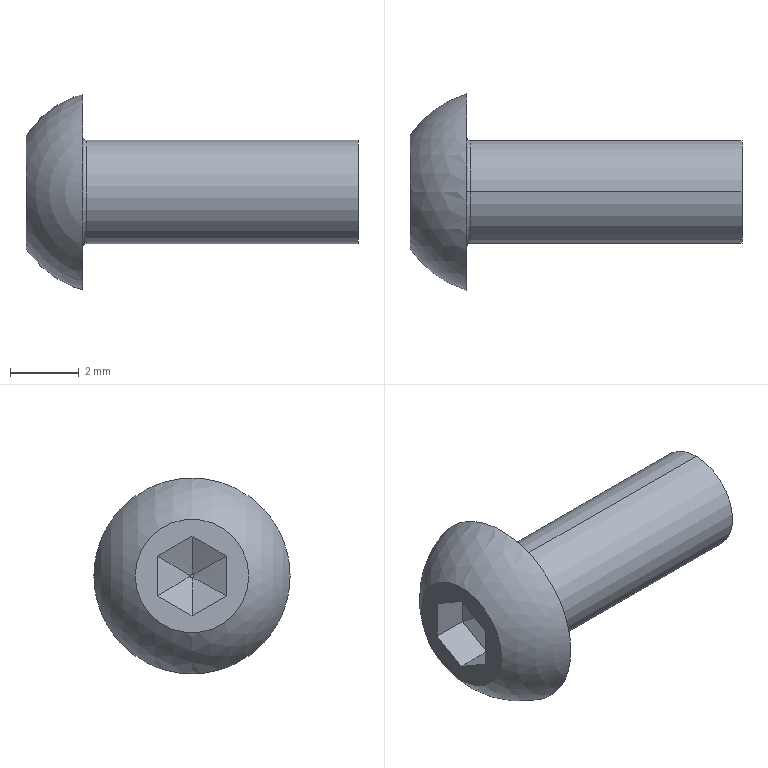Part | NX | features BREP 1 | 1 solid | 21 faces | box 9.65 x 5.7 x 5.7 mm | volume 82.821 mm3 | plane 10 | spline 6 | torus 2 | cylinder 2 | sphere 1 | commonest cylinder face diameters 3 x2
STEP:
#1=CARTESIAN_POINT('',(1.75,0.,1.5));
#2=VERTEX_POINT('',#1);
#3=CARTESIAN_POINT('',(1.75,0.,-1.5));
#4=VERTEX_POINT('',#3);
#5=CARTESIAN_POINT('',(1.75,0.,0.));
#6=DIRECTION('',(1.,0.,0.));
#7=DIRECTION('',(0.,0.,-1.));
#8=AXIS2_PLACEMENT_3D('',#5,#6,#7);
#9=CIRCLE('',#8,1.5);
#10=EDGE_CURVE('',#2,#4,#9,.T.);
#11=ORIENTED_EDGE('',*,*,#10,.F.);
#12=CARTESIAN_POINT('',(1.65,0.,1.6));
#13=VERTEX_POINT('',#12);
#14=CARTESIAN_POINT('',(1.75,0.,1.6));
#15=DIRECTION('',(0.,1.,0.));
#16=DIRECTION('',(0.,0.,1.));
#17=AXIS2_PLACEMENT_3D('',#14,#15,#16);
#18=CIRCLE('',#17,0.1);
#19=EDGE_CURVE('',#13,#2,#18,.F.);
#20=ORIENTED_EDGE('',*,*,#19,.F.);
#21=CARTESIAN_POINT('',(1.65,0.,-1.6));
#22=VERTEX_POINT('',#21);
#23=CARTESIAN_POINT('',(1.65,0.,0.));
#24=DIRECTION('',(-1.,0.,0.));
#25=DIRECTION('',(0.,0.,-1.));
#26=AXIS2_PLACEMENT_3D('',#23,#24,#25);
#27=CIRCLE('',#26,1.6);
#28=EDGE_CURVE('',#22,#13,#27,.T.);
#29=ORIENTED_EDGE('',*,*,#28,.F.);
#30=CARTESIAN_POINT('',(1.75,0.,-1.6));
#31=DIRECTION('',(0.,-1.,0.));
#32=DIRECTION('',(0.,0.,-1.));
#33=AXIS2_PLACEMENT_3D('',#30,#31,#32);
#34=CIRCLE('',#33,0.1);
#35=EDGE_CURVE('',#22,#4,#34,.F.);
#36=ORIENTED_EDGE('',*,*,#35,.T.);
#37=EDGE_LOOP('',(#11,#20,#29,#36));
#38=FACE_BOUND('',#37,.T.);
#39=CARTESIAN_POINT('',(1.75,0.,0.));
#40=DIRECTION('',(1.,0.,0.));
#41=DIRECTION('',(0.,0.,1.));
#42=AXIS2_PLACEMENT_3D('',#39,#40,#41);
#43=TOROIDAL_SURFACE('',#42,1.6,0.1);
#44=ADVANCED_FACE('',(#38),#43,.F.);
#45=CARTESIAN_POINT('',(9.65,0.,1.5));
#46=VERTEX_POINT('',#45);
#47=CARTESIAN_POINT('',(9.65,0.,-1.5));
#48=VERTEX_POINT('',#47);
#49=CARTESIAN_POINT('',(9.65,0.,0.));
#50=DIRECTION('',(-1.,0.,0.));
#51=DIRECTION('',(0.,0.,-1.));
#52=AXIS2_PLACEMENT_3D('',#49,#50,#51);
#53=CIRCLE('',#52,1.5);
#54=EDGE_CURVE('',#46,#48,#53,.T.);
#55=ORIENTED_EDGE('',*,*,#54,.T.);
#56=CARTESIAN_POINT('',(7.65,0.,-1.5));
#57=DIRECTION('',(-1.,0.,0.));
#58=VECTOR('',#57,1000.);
#59=LINE('',#56,#58);
#60=EDGE_CURVE('',#48,#4,#59,.T.);
#61=ORIENTED_EDGE('',*,*,#60,.T.);
#62=CARTESIAN_POINT('',(1.75,0.,0.));
#63=DIRECTION('',(1.,0.,0.));
#64=DIRECTION('',(0.,0.,-1.));
#65=AXIS2_PLACEMENT_3D('',#62,#63,#64);
#66=CIRCLE('',#65,1.5);
#67=EDGE_CURVE('',#4,#2,#66,.T.);
#68=ORIENTED_EDGE('',*,*,#67,.T.);
#69=CARTESIAN_POINT('',(7.65,0.,1.5));
#70=DIRECTION('',(-1.,0.,0.));
#71=VECTOR('',#70,1000.);
#72=LINE('',#69,#71);
#73=EDGE_CURVE('',#46,#2,#72,.T.);
#74=ORIENTED_EDGE('',*,*,#73,.F.);
#75=EDGE_LOOP('',(#55,#61,#68,#74));
#76=FACE_BOUND('',#75,.T.);
#77=CARTESIAN_POINT('',(7.65,0.,0.));
#78=DIRECTION('',(-1.,0.,0.));
#79=DIRECTION('',(0.,0.,-1.));
#80=AXIS2_PLACEMENT_3D('',#77,#78,#79);
#81=CYLINDRICAL_SURFACE('',#80,1.5);
#82=ADVANCED_FACE('',(#76),#81,.T.);
#83=CARTESIAN_POINT('',(1.65,2.85,0.));
#84=VERTEX_POINT('',#83);
#85=CARTESIAN_POINT('',(1.65,-2.85,0.));
#86=VERTEX_POINT('',#85);
#87=CARTESIAN_POINT('',(1.65,0.,0.));
#88=DIRECTION('',(1.,0.,0.));
#89=DIRECTION('',(0.,0.,-1.));
#90=AXIS2_PLACEMENT_3D('',#87,#88,#89);
#91=CIRCLE('',#90,2.85);
#92=EDGE_CURVE('',#84,#86,#91,.T.);
#93=ORIENTED_EDGE('',*,*,#92,.T.);
#94=CARTESIAN_POINT('',(1.65,0.,0.));
#95=DIRECTION('',(1.,0.,0.));
#96=DIRECTION('',(0.,0.,-1.));
#97=AXIS2_PLACEMENT_3D('',#94,#95,#96);
#98=CIRCLE('',#97,2.85);
#99=EDGE_CURVE('',#86,#84,#98,.T.);
#100=ORIENTED_EDGE('',*,*,#99,.T.);
#101=EDGE_LOOP('',(#93,#100));
#102=FACE_BOUND('',#101,.T.);
#103=ORIENTED_EDGE('',*,*,#28,.T.);
#104=CARTESIAN_POINT('',(1.65,0.,0.));
#105=DIRECTION('',(-1.,0.,0.));
#106=DIRECTION('',(0.,0.,-1.));
#107=AXIS2_PLACEMENT_3D('',#104,#105,#106);
#108=CIRCLE('',#107,1.6);
#109=EDGE_CURVE('',#13,#22,#108,.T.);
#110=ORIENTED_EDGE('',*,*,#109,.T.);
#111=EDGE_LOOP('',(#103,#110));
#112=FACE_BOUND('',#111,.T.);
#113=CARTESIAN_POINT('',(1.65,0.,0.));
#114=DIRECTION('',(1.,0.,0.));
#115=DIRECTION('',(0.,-1.,0.));
#116=AXIS2_PLACEMENT_3D('',#113,#114,#115);
#117=PLANE('',#116);
#118=ADVANCED_FACE('',(#102,#112),#117,.T.);
#119=ORIENTED_EDGE('',*,*,#92,.F.);
#120=ORIENTED_EDGE('',*,*,#99,.F.);
#121=EDGE_LOOP('',(#119,#120));
#122=FACE_BOUND('',#121,.T.);
#123=CARTESIAN_POINT('',(0.,1.65,0.));
#124=VERTEX_POINT('',#123);
#125=CARTESIAN_POINT('',(0.,-1.65,0.));
#126=VERTEX_POINT('',#125);
#127=CARTESIAN_POINT('',(0.,0.,0.));
#128=DIRECTION('',(1.,0.,0.));
#129=DIRECTION('',(0.,0.,-1.));
#130=AXIS2_PLACEMENT_3D('',#127,#128,#129);
#131=CIRCLE('',#130,1.65);
#132=EDGE_CURVE('',#124,#126,#131,.T.);
#133=ORIENTED_EDGE('',*,*,#132,.T.);
#134=CARTESIAN_POINT('',(0.,0.,0.));
#135=DIRECTION('',(1.,0.,0.));
#136=DIRECTION('',(0.,0.,-1.));
#137=AXIS2_PLACEMENT_3D('',#134,#135,#136);
#138=CIRCLE('',#137,1.65);
#139=EDGE_CURVE('',#126,#124,#138,.T.);
#140=ORIENTED_EDGE('',*,*,#139,.T.);
#141=EDGE_LOOP('',(#133,#140));
#142=FACE_BOUND('',#141,.T.);
#143=CARTESIAN_POINT('',(2.461,0.,0.));
#144=DIRECTION('',(0.,1.,0.));
#145=DIRECTION('',(-0.2585,0.,-0.966));
#146=AXIS2_PLACEMENT_3D('',#143,#144,#145);
#147=SPHERICAL_SURFACE('',#146,2.963);
#148=ADVANCED_FACE('',(#122,#142),#147,.T.);
#149=ORIENTED_EDGE('',*,*,#132,.F.);
#150=ORIENTED_EDGE('',*,*,#139,.F.);
#151=EDGE_LOOP('',(#149,#150));
#152=FACE_BOUND('',#151,.T.);
#153=CARTESIAN_POINT('',(0.,1.,-0.5774));
#154=VERTEX_POINT('',#153);
#155=CARTESIAN_POINT('',(0.,0.,-1.155));
#156=VERTEX_POINT('',#155);
#157=CARTESIAN_POINT('',(0.,1.,-0.5774));
#158=DIRECTION('',(0.,-0.866,-0.5));
#159=VECTOR('',#158,1000.);
#160=LINE('',#157,#159);
#161=EDGE_CURVE('',#154,#156,#160,.T.);
#162=ORIENTED_EDGE('',*,*,#161,.F.);
#163=CARTESIAN_POINT('',(0.,1.,0.5774));
#164=VERTEX_POINT('',#163);
#165=CARTESIAN_POINT('',(0.,1.,0.));
#166=DIRECTION('',(0.,0.,-1.));
#167=VECTOR('',#166,1000.);
#168=LINE('',#165,#167);
#169=EDGE_CURVE('',#164,#154,#168,.T.);
#170=ORIENTED_EDGE('',*,*,#169,.F.);
#171=CARTESIAN_POINT('',(0.,0.,1.155));
#172=VERTEX_POINT('',#171);
#173=CARTESIAN_POINT('',(0.,0.,1.155));
#174=DIRECTION('',(0.,0.866,-0.5));
#175=VECTOR('',#174,1000.);
#176=LINE('',#173,#175);
#177=EDGE_CURVE('',#172,#164,#176,.T.);
#178=ORIENTED_EDGE('',*,*,#177,.F.);
#179=CARTESIAN_POINT('',(0.,-1.,0.5774));
#180=VERTEX_POINT('',#179);
#181=CARTESIAN_POINT('',(0.,-1.,0.5774));
#182=DIRECTION('',(0.,0.866,0.5));
#183=VECTOR('',#182,1000.);
#184=LINE('',#181,#183);
#185=EDGE_CURVE('',#180,#172,#184,.T.);
#186=ORIENTED_EDGE('',*,*,#185,.F.);
#187=CARTESIAN_POINT('',(0.,-1.,-0.5774));
#188=VERTEX_POINT('',#187);
#189=CARTESIAN_POINT('',(0.,-1.,0.));
#190=DIRECTION('',(0.,0.,1.));
#191=VECTOR('',#190,1000.);
#192=LINE('',#189,#191);
#193=EDGE_CURVE('',#188,#180,#192,.T.);
#194=ORIENTED_EDGE('',*,*,#193,.F.);
#195=CARTESIAN_POINT('',(0.,0.,-1.155));
#196=DIRECTION('',(0.,-0.866,0.5));
#197=VECTOR('',#196,1000.);
#198=LINE('',#195,#197);
#199=EDGE_CURVE('',#156,#188,#198,.T.);
#200=ORIENTED_EDGE('',*,*,#199,.F.);
#201=EDGE_LOOP('',(#162,#170,#178,#186,#194,#200));
#202=FACE_BOUND('',#201,.T.);
#203=CARTESIAN_POINT('',(0.,0.,0.));
#204=DIRECTION('',(1.,0.,0.));
#205=DIRECTION('',(0.,-1.,0.));
#206=AXIS2_PLACEMENT_3D('',#203,#204,#205);
#207=PLANE('',#206);
#208=ADVANCED_FACE('',(#152,#202),#207,.F.);
#209=CARTESIAN_POINT('',(1.04,-1.,-0.5774));
#210=VERTEX_POINT('',#209);
#211=CARTESIAN_POINT('',(1.04,0.,-1.155));
#212=VERTEX_POINT('',#211);
#213=CARTESIAN_POINT('',(1.04,-1.,-0.5774));
#214=DIRECTION('',(0.,0.866,-0.5));
#215=VECTOR('',#214,1000.);
#216=LINE('',#213,#215);
#217=EDGE_CURVE('',#210,#212,#216,.T.);
#218=ORIENTED_EDGE('',*,*,#217,.T.);
#219=CARTESIAN_POINT('',(1.04,0.,-1.155));
#220=DIRECTION('',(-1.,0.,0.));
#221=VECTOR('',#220,1000.);
#222=LINE('',#219,#221);
#223=EDGE_CURVE('',#212,#156,#222,.T.);
#224=ORIENTED_EDGE('',*,*,#223,.T.);
#225=ORIENTED_EDGE('',*,*,#199,.T.);
#226=CARTESIAN_POINT('',(1.04,-1.,-0.5774));
#227=DIRECTION('',(1.,0.,0.));
#228=VECTOR('',#227,1000.);
#229=LINE('',#226,#228);
#230=EDGE_CURVE('',#188,#210,#229,.T.);
#231=ORIENTED_EDGE('',*,*,#230,.T.);
#232=EDGE_LOOP('',(#218,#224,#225,#231));
#233=FACE_BOUND('',#232,.T.);
#234=CARTESIAN_POINT('',(1.04,-1.,-0.5774));
#235=DIRECTION('',(0.,0.5,0.866));
#236=DIRECTION('',(-1.,0.,0.));
#237=AXIS2_PLACEMENT_3D('',#234,#235,#236);
#238=PLANE('',#237);
#239=ADVANCED_FACE('',(#233),#238,.T.);
#240=CARTESIAN_POINT('',(1.04,1.,-0.5774));
#241=VERTEX_POINT('',#240);
#242=CARTESIAN_POINT('',(1.04,0.,-1.155));
#243=DIRECTION('',(0.,0.866,0.5));
#244=VECTOR('',#243,1000.);
#245=LINE('',#242,#244);
#246=EDGE_CURVE('',#212,#241,#245,.T.);
#247=ORIENTED_EDGE('',*,*,#246,.T.);
#248=CARTESIAN_POINT('',(1.04,1.,-0.5774));
#249=DIRECTION('',(-1.,0.,0.));
#250=VECTOR('',#249,1000.);
#251=LINE('',#248,#250);
#252=EDGE_CURVE('',#241,#154,#251,.T.);
#253=ORIENTED_EDGE('',*,*,#252,.T.);
#254=ORIENTED_EDGE('',*,*,#161,.T.);
#255=ORIENTED_EDGE('',*,*,#223,.F.);
#256=EDGE_LOOP('',(#247,#253,#254,#255));
#257=FACE_BOUND('',#256,.T.);
#258=CARTESIAN_POINT('',(1.04,0.,-1.155));
#259=DIRECTION('',(0.,-0.5,0.866));
#260=DIRECTION('',(1.,0.,0.));
#261=AXIS2_PLACEMENT_3D('',#258,#259,#260);
#262=PLANE('',#261);
#263=ADVANCED_FACE('',(#257),#262,.T.);
#264=CARTESIAN_POINT('',(1.04,1.,0.5774));
#265=VERTEX_POINT('',#264);
#266=CARTESIAN_POINT('',(1.04,1.,-0.5774));
#267=DIRECTION('',(0.,0.,1.));
#268=VECTOR('',#267,1000.);
#269=LINE('',#266,#268);
#270=EDGE_CURVE('',#241,#265,#269,.T.);
#271=ORIENTED_EDGE('',*,*,#270,.T.);
#272=CARTESIAN_POINT('',(1.04,1.,0.5774));
#273=DIRECTION('',(-1.,0.,0.));
#274=VECTOR('',#273,1000.);
#275=LINE('',#272,#274);
#276=EDGE_CURVE('',#265,#164,#275,.T.);
#277=ORIENTED_EDGE('',*,*,#276,.T.);
#278=ORIENTED_EDGE('',*,*,#169,.T.);
#279=ORIENTED_EDGE('',*,*,#252,.F.);
#280=EDGE_LOOP('',(#271,#277,#278,#279));
#281=FACE_BOUND('',#280,.T.);
#282=CARTESIAN_POINT('',(1.04,1.,-0.5774));
#283=DIRECTION('',(0.,-1.,0.));
#284=DIRECTION('',(1.,0.,0.));
#285=AXIS2_PLACEMENT_3D('',#282,#283,#284);
#286=PLANE('',#285);
#287=ADVANCED_FACE('',(#281),#286,.T.);
#288=CARTESIAN_POINT('',(1.04,0.,1.155));
#289=VERTEX_POINT('',#288);
#290=CARTESIAN_POINT('',(1.04,1.,0.5774));
#291=DIRECTION('',(0.,-0.866,0.5));
#292=VECTOR('',#291,1000.);
#293=LINE('',#290,#292);
#294=EDGE_CURVE('',#265,#289,#293,.T.);
#295=ORIENTED_EDGE('',*,*,#294,.T.);
#296=CARTESIAN_POINT('',(1.04,0.,1.155));
#297=DIRECTION('',(-1.,0.,0.));
#298=VECTOR('',#297,1000.);
#299=LINE('',#296,#298);
#300=EDGE_CURVE('',#289,#172,#299,.T.);
#301=ORIENTED_EDGE('',*,*,#300,.T.);
#302=ORIENTED_EDGE('',*,*,#177,.T.);
#303=ORIENTED_EDGE('',*,*,#276,.F.);
#304=EDGE_LOOP('',(#295,#301,#302,#303));
#305=FACE_BOUND('',#304,.T.);
#306=CARTESIAN_POINT('',(1.04,1.,0.5774));
#307=DIRECTION('',(0.,-0.5,-0.866));
#308=DIRECTION('',(0.,0.866,-0.5));
#309=AXIS2_PLACEMENT_3D('',#306,#307,#308);
#310=PLANE('',#309);
#311=ADVANCED_FACE('',(#305),#310,.T.);
#312=CARTESIAN_POINT('',(1.04,-1.,0.5774));
#313=VERTEX_POINT('',#312);
#314=CARTESIAN_POINT('',(1.04,0.,1.155));
#315=DIRECTION('',(0.,-0.866,-0.5));
#316=VECTOR('',#315,1000.);
#317=LINE('',#314,#316);
#318=EDGE_CURVE('',#289,#313,#317,.T.);
#319=ORIENTED_EDGE('',*,*,#318,.T.);
#320=CARTESIAN_POINT('',(1.04,-1.,0.5774));
#321=DIRECTION('',(-1.,0.,0.));
#322=VECTOR('',#321,1000.);
#323=LINE('',#320,#322);
#324=EDGE_CURVE('',#313,#180,#323,.T.);
#325=ORIENTED_EDGE('',*,*,#324,.T.);
#326=ORIENTED_EDGE('',*,*,#185,.T.);
#327=ORIENTED_EDGE('',*,*,#300,.F.);
#328=EDGE_LOOP('',(#319,#325,#326,#327));
#329=FACE_BOUND('',#328,.T.);
#330=CARTESIAN_POINT('',(1.04,0.,1.155));
#331=DIRECTION('',(0.,0.5,-0.866));
#332=DIRECTION('',(1.,0.,0.));
#333=AXIS2_PLACEMENT_3D('',#330,#331,#332);
#334=PLANE('',#333);
#335=ADVANCED_FACE('',(#329),#334,.T.);
#336=CARTESIAN_POINT('',(1.04,-1.,0.5774));
#337=DIRECTION('',(0.,0.,-1.));
#338=VECTOR('',#337,1000.);
#339=LINE('',#336,#338);
#340=EDGE_CURVE('',#313,#210,#339,.T.);
#341=ORIENTED_EDGE('',*,*,#340,.T.);
#342=ORIENTED_EDGE('',*,*,#230,.F.);
#343=ORIENTED_EDGE('',*,*,#193,.T.);
#344=ORIENTED_EDGE('',*,*,#324,.F.);
#345=EDGE_LOOP('',(#341,#342,#343,#344));
#346=FACE_BOUND('',#345,.T.);
#347=CARTESIAN_POINT('',(1.04,-1.,0.5774));
#348=DIRECTION('',(0.,1.,0.));
#349=DIRECTION('',(-1.,0.,0.));
#350=AXIS2_PLACEMENT_3D('',#347,#348,#349);
#351=PLANE('',#350);
#352=ADVANCED_FACE('',(#346),#351,.T.);
#353=CARTESIAN_POINT('',(1.542,-0.022,-0.0381));
#354=VERTEX_POINT('',#353);
#355=CARTESIAN_POINT('',(1.04,-1.,-0.5774));
#356=CARTESIAN_POINT('',(1.121,-0.845,-0.4878));
#357=CARTESIAN_POINT('',(1.204,-0.6803,-0.3988));
#358=CARTESIAN_POINT('',(1.372,-0.3525,-0.2177));
#359=CARTESIAN_POINT('',(1.399,-0.3014,-0.1869));
#360=CARTESIAN_POINT('',(1.526,-0.0494,-0.05698));
#361=CARTESIAN_POINT('',(1.541,-0.0292,-0.03808));
#362=CARTESIAN_POINT('',(1.543,-0.02217,-0.0384));
#363=B_SPLINE_CURVE_WITH_KNOTS('',3,(#355,#356,#357,#358,#359,#360,#361,#362),.UNSPECIFIED.,.F.,.F.,(4,1,1,1,1,4),(0.,0.5,0.625,0.75,0.875,1.),.UNSPECIFIED.);
#364=EDGE_CURVE('',#354,#210,#363,.F.);
#365=ORIENTED_EDGE('',*,*,#364,.F.);
#366=CARTESIAN_POINT('',(1.543,-0.02217,-0.0384));
#367=CARTESIAN_POINT('',(1.546,-0.01126,-0.03849));
#368=CARTESIAN_POINT('',(1.469,-0.02,-0.1962));
#369=CARTESIAN_POINT('',(1.414,-0.01237,-0.3217));
#370=CARTESIAN_POINT('',(1.369,-0.01206,-0.4203));
#371=CARTESIAN_POINT('',(1.257,-0.007308,-0.6718));
#372=CARTESIAN_POINT('',(1.2,-0.005747,-0.7972));
#373=CARTESIAN_POINT('',(1.095,-0.001899,-1.032));
#374=CARTESIAN_POINT('',(1.04,0.,-1.155));
#375=B_SPLINE_CURVE_WITH_KNOTS('',3,(#366,#367,#368,#369,#370,#371,#372,#373,#374),.UNSPECIFIED.,.F.,.F.,(4,1,1,1,1,1,4),(0.,0.125,0.25,0.375,0.5,0.75,1.),.UNSPECIFIED.);
#376=EDGE_CURVE('',#212,#354,#375,.F.);
#377=ORIENTED_EDGE('',*,*,#376,.F.);
#378=ORIENTED_EDGE('',*,*,#217,.F.);
#379=EDGE_LOOP('',(#365,#377,#378));
#380=FACE_BOUND('',#379,.T.);
#381=CARTESIAN_POINT('',(1.04,-1.,-0.5774));
#382=CARTESIAN_POINT('',(1.207,-0.6811,-0.3932));
#383=CARTESIAN_POINT('',(1.373,-0.3622,-0.2091));
#384=CARTESIAN_POINT('',(1.542,-0.04011,-0.02316));
#385=CARTESIAN_POINT('',(1.543,-0.03692,-0.02132));
#386=CARTESIAN_POINT('',(1.545,-0.03373,-0.01948));
#387=CARTESIAN_POINT('',(1.04,-0.8333,-0.6736));
#388=CARTESIAN_POINT('',(1.207,-0.5686,-0.4598));
#389=CARTESIAN_POINT('',(1.373,-0.3039,-0.246));
#390=CARTESIAN_POINT('',(1.542,-0.03649,-0.03008));
#391=CARTESIAN_POINT('',(1.543,-0.03384,-0.02794));
#392=CARTESIAN_POINT('',(1.545,-0.03119,-0.0258));
#393=CARTESIAN_POINT('',(1.04,-0.6667,-0.7698));
#394=CARTESIAN_POINT('',(1.207,-0.4553,-0.526));
#395=CARTESIAN_POINT('',(1.373,-0.2439,-0.2822));
#396=CARTESIAN_POINT('',(1.542,-0.03036,-0.03603));
#397=CARTESIAN_POINT('',(1.543,-0.02825,-0.03359));
#398=CARTESIAN_POINT('',(1.545,-0.02613,-0.03115));
#399=CARTESIAN_POINT('',(1.04,-0.3333,-0.9623));
#400=CARTESIAN_POINT('',(1.207,-0.2279,-0.6573));
#401=CARTESIAN_POINT('',(1.373,-0.1225,-0.3523));
#402=CARTESIAN_POINT('',(1.542,-0.01602,-0.04431));
#403=CARTESIAN_POINT('',(1.543,-0.01497,-0.04126));
#404=CARTESIAN_POINT('',(1.545,-0.01391,-0.03821));
#405=CARTESIAN_POINT('',(1.04,-0.1667,-1.058));
#406=CARTESIAN_POINT('',(1.207,-0.1139,-0.7223));
#407=CARTESIAN_POINT('',(1.373,-0.06111,-0.3862));
#408=CARTESIAN_POINT('',(1.542,-0.007806,-0.04664));
#409=CARTESIAN_POINT('',(1.543,-0.007278,-0.04328));
#410=CARTESIAN_POINT('',(1.545,-0.00675,-0.03992));
#411=CARTESIAN_POINT('',(1.04,0.,-1.155));
#412=CARTESIAN_POINT('',(1.207,0.,-0.7865));
#413=CARTESIAN_POINT('',(1.373,0.,-0.4182));
#414=CARTESIAN_POINT('',(1.542,0.,-0.04632));
#415=CARTESIAN_POINT('',(1.543,0.,-0.04264));
#416=CARTESIAN_POINT('',(1.545,0.,-0.03895));
#417=B_SPLINE_SURFACE_WITH_KNOTS('',3,3,((#381,#382,#383,#384,#385,#386),(#387,#388,#389,#390,#391,#392),(#393,#394,#395,#396,#397,#398),(#399,#400,#401,#402,#403,#404),(#405,#406,#407,#408,#409,#410),(#411,#412,#413,#414,#415,#416)),.RULED_SURF.,.F.,.F.,.F.,(4,2,4),(4,2,4),(0.,0.5,1.),(0.,0.9901,1.),.UNSPECIFIED.);
#418=ADVANCED_FACE('',(#380),#417,.F.);
#419=ORIENTED_EDGE('',*,*,#376,.T.);
#420=CARTESIAN_POINT('',(1.542,0.04399,0.));
#421=VERTEX_POINT('',#420);
#422=CARTESIAN_POINT('',(1.54,0.04399,0.));
#423=CARTESIAN_POINT('',(1.54,0.05112,-0.03859));
#424=CARTESIAN_POINT('',(1.54,0.008464,-0.06403));
#425=CARTESIAN_POINT('',(1.54,-0.022,-0.0381));
#426=B_SPLINE_CURVE_WITH_KNOTS('',3,(#422,#423,#424,#425),.UNSPECIFIED.,.F.,.F.,(4,4),(0.,1.),.UNSPECIFIED.);
#427=EDGE_CURVE('',#421,#354,#426,.T.);
#428=ORIENTED_EDGE('',*,*,#427,.F.);
#429=CARTESIAN_POINT('',(1.544,0.04448,-0.0005402));
#430=CARTESIAN_POINT('',(1.543,0.04731,-0.00108));
#431=CARTESIAN_POINT('',(1.528,0.0899,-0.02055));
#432=CARTESIAN_POINT('',(1.432,0.2651,-0.1353));
#433=CARTESIAN_POINT('',(1.403,0.3189,-0.1671));
#434=CARTESIAN_POINT('',(1.278,0.5543,-0.3097));
#435=CARTESIAN_POINT('',(1.253,0.6008,-0.3374));
#436=CARTESIAN_POINT('',(1.167,0.7617,-0.4341));
#437=CARTESIAN_POINT('',(1.096,0.8947,-0.5141));
#438=CARTESIAN_POINT('',(1.04,1.,-0.5774));
#439=B_SPLINE_CURVE_WITH_KNOTS('',3,(#429,#430,#431,#432,#433,#434,#435,#436,#437,#438),.UNSPECIFIED.,.F.,.F.,(4,1,1,1,1,1,1,4),(0.,0.125,0.25,0.375,0.5,0.625,0.75,1.),.UNSPECIFIED.);
#440=EDGE_CURVE('',#241,#421,#439,.F.);
#441=ORIENTED_EDGE('',*,*,#440,.F.);
#442=ORIENTED_EDGE('',*,*,#246,.F.);
#443=EDGE_LOOP('',(#419,#428,#441,#442));
#444=FACE_BOUND('',#443,.T.);
#445=CARTESIAN_POINT('',(1.04,-0.5135,-1.451));
#446=CARTESIAN_POINT('',(1.207,-0.3509,-0.9841));
#447=CARTESIAN_POINT('',(1.373,-0.1883,-0.5171));
#448=CARTESIAN_POINT('',(1.542,-0.02405,-0.04533));
#449=CARTESIAN_POINT('',(1.543,-0.02242,-0.04066));
#450=CARTESIAN_POINT('',(1.545,-0.0208,-0.03599));
#451=CARTESIAN_POINT('',(1.04,-0.3423,-1.352));
#452=CARTESIAN_POINT('',(1.207,-0.2339,-0.9182));
#453=CARTESIAN_POINT('',(1.373,-0.1255,-0.4841));
#454=CARTESIAN_POINT('',(1.542,-0.01603,-0.04566));
#455=CARTESIAN_POINT('',(1.543,-0.01495,-0.04132));
#456=CARTESIAN_POINT('',(1.545,-0.01386,-0.03698));
#457=CARTESIAN_POINT('',(1.04,-0.1712,-1.254));
#458=CARTESIAN_POINT('',(1.207,-0.117,-0.8523));
#459=CARTESIAN_POINT('',(1.373,-0.06276,-0.4512));
#460=CARTESIAN_POINT('',(1.542,-0.008016,-0.04599));
#461=CARTESIAN_POINT('',(1.543,-0.007474,-0.04198));
#462=CARTESIAN_POINT('',(1.545,-0.006932,-0.03796));
#463=CARTESIAN_POINT('',(1.04,0.1667,-1.058));
#464=CARTESIAN_POINT('',(1.207,0.1139,-0.7223));
#465=CARTESIAN_POINT('',(1.373,0.06111,-0.3862));
#466=CARTESIAN_POINT('',(1.542,0.007806,-0.04664));
#467=CARTESIAN_POINT('',(1.543,0.007278,-0.04328));
#468=CARTESIAN_POINT('',(1.545,0.00675,-0.03992));
#469=CARTESIAN_POINT('',(1.04,0.3333,-0.9623));
#470=CARTESIAN_POINT('',(1.207,0.2279,-0.6573));
#471=CARTESIAN_POINT('',(1.373,0.1225,-0.3523));
#472=CARTESIAN_POINT('',(1.542,0.01602,-0.04431));
#473=CARTESIAN_POINT('',(1.543,0.01497,-0.04126));
#474=CARTESIAN_POINT('',(1.545,0.01391,-0.03821));
#475=CARTESIAN_POINT('',(1.04,0.6667,-0.7698));
#476=CARTESIAN_POINT('',(1.207,0.4553,-0.526));
#477=CARTESIAN_POINT('',(1.373,0.2439,-0.2822));
#478=CARTESIAN_POINT('',(1.542,0.03036,-0.03603));
#479=CARTESIAN_POINT('',(1.543,0.02825,-0.03359));
#480=CARTESIAN_POINT('',(1.545,0.02613,-0.03115));
#481=CARTESIAN_POINT('',(1.04,0.8333,-0.6736));
#482=CARTESIAN_POINT('',(1.207,0.5686,-0.4598));
#483=CARTESIAN_POINT('',(1.373,0.3039,-0.246));
#484=CARTESIAN_POINT('',(1.542,0.03649,-0.03008));
#485=CARTESIAN_POINT('',(1.543,0.03384,-0.02794));
#486=CARTESIAN_POINT('',(1.545,0.03119,-0.0258));
#487=CARTESIAN_POINT('',(1.04,1.171,-0.4785));
#488=CARTESIAN_POINT('',(1.207,0.7966,-0.3249));
#489=CARTESIAN_POINT('',(1.373,0.4221,-0.1712));
#490=CARTESIAN_POINT('',(1.542,0.04384,-0.01605));
#491=CARTESIAN_POINT('',(1.543,0.04009,-0.01452));
#492=CARTESIAN_POINT('',(1.545,0.03634,-0.01298));
#493=CARTESIAN_POINT('',(1.04,1.342,-0.3797));
#494=CARTESIAN_POINT('',(1.207,0.9122,-0.2565));
#495=CARTESIAN_POINT('',(1.373,0.482,-0.1334));
#496=CARTESIAN_POINT('',(1.542,0.04756,-0.008945));
#497=CARTESIAN_POINT('',(1.543,0.04326,-0.007713));
#498=CARTESIAN_POINT('',(1.545,0.03895,-0.006482));
#499=CARTESIAN_POINT('',(1.04,1.513,-0.2809));
#500=CARTESIAN_POINT('',(1.207,1.028,-0.1882));
#501=CARTESIAN_POINT('',(1.373,0.5419,-0.09547));
#502=CARTESIAN_POINT('',(1.542,0.05128,-0.001838));
#503=CARTESIAN_POINT('',(1.543,0.04642,-0.0009111));
#504=CARTESIAN_POINT('',(1.545,0.04156,0.00001596));
#505=B_SPLINE_SURFACE_WITH_KNOTS('',3,3,((#445,#446,#447,#448,#449,#450),(#451,#452,#453,#454,#455,#456),(#457,#458,#459,#460,#461,#462),(#463,#464,#465,#466,#467,#468),(#469,#470,#471,#472,#473,#474),(#475,#476,#477,#478,#479,#480),(#481,#482,#483,#484,#485,#486),(#487,#488,#489,#490,#491,#492),(#493,#494,#495,#496,#497,#498),(#499,#500,#501,#502,#503,#504)),.RULED_SURF.,.F.,.F.,.F.,(4,2,2,2,4),(4,2,4),(0.,0.2533,0.5,0.7467,1.),(0.,0.9901,1.),.UNSPECIFIED.);
#506=ADVANCED_FACE('',(#444),#505,.F.);
#507=ORIENTED_EDGE('',*,*,#440,.T.);
#508=CARTESIAN_POINT('',(1.543,0.04434,0.));
#509=CARTESIAN_POINT('',(1.546,0.03897,0.009492));
#510=CARTESIAN_POINT('',(1.469,0.1799,0.08079));
#511=CARTESIAN_POINT('',(1.414,0.2848,0.1501));
#512=CARTESIAN_POINT('',(1.369,0.3701,0.1997));
#513=CARTESIAN_POINT('',(1.257,0.5855,0.3296));
#514=CARTESIAN_POINT('',(1.2,0.6932,0.3936));
#515=CARTESIAN_POINT('',(1.095,0.8945,0.5143));
#516=CARTESIAN_POINT('',(1.04,1.,0.5774));
#517=B_SPLINE_CURVE_WITH_KNOTS('',3,(#508,#509,#510,#511,#512,#513,#514,#515,#516),.UNSPECIFIED.,.F.,.F.,(4,1,1,1,1,1,4),(0.,0.125,0.25,0.375,0.5,0.75,1.),.UNSPECIFIED.);
#518=EDGE_CURVE('',#265,#421,#517,.F.);
#519=ORIENTED_EDGE('',*,*,#518,.F.);
#520=ORIENTED_EDGE('',*,*,#270,.F.);
#521=EDGE_LOOP('',(#507,#519,#520));
#522=FACE_BOUND('',#521,.T.);
#523=CARTESIAN_POINT('',(1.04,1.,-0.5774));
#524=CARTESIAN_POINT('',(1.207,0.6811,-0.3932));
#525=CARTESIAN_POINT('',(1.373,0.3622,-0.2091));
#526=CARTESIAN_POINT('',(1.542,0.04011,-0.02316));
#527=CARTESIAN_POINT('',(1.543,0.03692,-0.02132));
#528=CARTESIAN_POINT('',(1.545,0.03373,-0.01948));
#529=CARTESIAN_POINT('',(1.04,1.,-0.3849));
#530=CARTESIAN_POINT('',(1.207,0.6825,-0.2625));
#531=CARTESIAN_POINT('',(1.373,0.365,-0.1402));
#532=CARTESIAN_POINT('',(1.542,0.04429,-0.01656));
#533=CARTESIAN_POINT('',(1.543,0.04112,-0.01534));
#534=CARTESIAN_POINT('',(1.545,0.03794,-0.01411));
#535=CARTESIAN_POINT('',(1.04,1.,-0.1925));
#536=CARTESIAN_POINT('',(1.207,0.6832,-0.1313));
#537=CARTESIAN_POINT('',(1.373,0.3664,-0.07008));
#538=CARTESIAN_POINT('',(1.542,0.04638,-0.00828));
#539=CARTESIAN_POINT('',(1.543,0.04321,-0.007668));
#540=CARTESIAN_POINT('',(1.545,0.04005,-0.007056));
#541=CARTESIAN_POINT('',(1.04,1.,0.1925));
#542=CARTESIAN_POINT('',(1.207,0.6832,0.1313));
#543=CARTESIAN_POINT('',(1.373,0.3664,0.07008));
#544=CARTESIAN_POINT('',(1.542,0.04638,0.00828));
#545=CARTESIAN_POINT('',(1.543,0.04321,0.007668));
#546=CARTESIAN_POINT('',(1.545,0.04005,0.007056));
#547=CARTESIAN_POINT('',(1.04,1.,0.3849));
#548=CARTESIAN_POINT('',(1.207,0.6825,0.2625));
#549=CARTESIAN_POINT('',(1.373,0.365,0.1402));
#550=CARTESIAN_POINT('',(1.542,0.04429,0.01656));
#551=CARTESIAN_POINT('',(1.543,0.04112,0.01534));
#552=CARTESIAN_POINT('',(1.545,0.03794,0.01411));
#553=CARTESIAN_POINT('',(1.04,1.,0.5774));
#554=CARTESIAN_POINT('',(1.207,0.6811,0.3932));
#555=CARTESIAN_POINT('',(1.373,0.3622,0.2091));
#556=CARTESIAN_POINT('',(1.542,0.04011,0.02316));
#557=CARTESIAN_POINT('',(1.543,0.03692,0.02132));
#558=CARTESIAN_POINT('',(1.545,0.03373,0.01948));
#559=B_SPLINE_SURFACE_WITH_KNOTS('',3,3,((#523,#524,#525,#526,#527,#528),(#529,#530,#531,#532,#533,#534),(#535,#536,#537,#538,#539,#540),(#541,#542,#543,#544,#545,#546),(#547,#548,#549,#550,#551,#552),(#553,#554,#555,#556,#557,#558)),.RULED_SURF.,.F.,.F.,.F.,(4,2,4),(4,2,4),(0.,0.5,1.),(0.,0.9901,1.),.UNSPECIFIED.);
#560=ADVANCED_FACE('',(#522),#559,.F.);
#561=ORIENTED_EDGE('',*,*,#518,.T.);
#562=CARTESIAN_POINT('',(1.542,-0.022,0.0381));
#563=VERTEX_POINT('',#562);
#564=CARTESIAN_POINT('',(1.54,-0.022,0.0381));
#565=CARTESIAN_POINT('',(1.54,0.007863,0.06357));
#566=CARTESIAN_POINT('',(1.54,0.05122,0.03935));
#567=CARTESIAN_POINT('',(1.54,0.04399,0.));
#568=B_SPLINE_CURVE_WITH_KNOTS('',3,(#564,#565,#566,#567),.UNSPECIFIED.,.F.,.F.,(4,4),(0.,1.),.UNSPECIFIED.);
#569=EDGE_CURVE('',#563,#421,#568,.T.);
#570=ORIENTED_EDGE('',*,*,#569,.F.);
#571=CARTESIAN_POINT('',(1.544,-0.02177,0.03879));
#572=CARTESIAN_POINT('',(1.543,-0.02272,0.04151));
#573=CARTESIAN_POINT('',(1.528,-0.02716,0.08813));
#574=CARTESIAN_POINT('',(1.432,-0.01539,0.2973));
#575=CARTESIAN_POINT('',(1.403,-0.01471,0.3598));
#576=CARTESIAN_POINT('',(1.278,-0.008951,0.6349));
#577=CARTESIAN_POINT('',(1.253,-0.008241,0.689));
#578=CARTESIAN_POINT('',(1.167,-0.004903,0.8767));
#579=CARTESIAN_POINT('',(1.096,-0.002132,1.032));
#580=CARTESIAN_POINT('',(1.04,0.,1.155));
#581=B_SPLINE_CURVE_WITH_KNOTS('',3,(#571,#572,#573,#574,#575,#576,#577,#578,#579,#580),.UNSPECIFIED.,.F.,.F.,(4,1,1,1,1,1,1,4),(0.,0.125,0.25,0.375,0.5,0.625,0.75,1.),.UNSPECIFIED.);
#582=EDGE_CURVE('',#289,#563,#581,.F.);
#583=ORIENTED_EDGE('',*,*,#582,.F.);
#584=ORIENTED_EDGE('',*,*,#294,.F.);
#585=EDGE_LOOP('',(#561,#570,#583,#584));
#586=FACE_BOUND('',#585,.T.);
#587=CARTESIAN_POINT('',(1.04,1.513,0.2809));
#588=CARTESIAN_POINT('',(1.207,1.028,0.1882));
#589=CARTESIAN_POINT('',(1.373,0.5419,0.09547));
#590=CARTESIAN_POINT('',(1.542,0.05128,0.001838));
#591=CARTESIAN_POINT('',(1.543,0.04642,0.0009111));
#592=CARTESIAN_POINT('',(1.545,0.04156,-0.00001596));
#593=CARTESIAN_POINT('',(1.04,1.342,0.3797));
#594=CARTESIAN_POINT('',(1.207,0.9122,0.2565));
#595=CARTESIAN_POINT('',(1.373,0.482,0.1334));
#596=CARTESIAN_POINT('',(1.542,0.04756,0.008945));
#597=CARTESIAN_POINT('',(1.543,0.04326,0.007713));
#598=CARTESIAN_POINT('',(1.545,0.03895,0.006482));
#599=CARTESIAN_POINT('',(1.04,1.171,0.4785));
#600=CARTESIAN_POINT('',(1.207,0.7966,0.3249));
#601=CARTESIAN_POINT('',(1.373,0.4221,0.1712));
#602=CARTESIAN_POINT('',(1.542,0.04384,0.01605));
#603=CARTESIAN_POINT('',(1.543,0.04009,0.01452));
#604=CARTESIAN_POINT('',(1.545,0.03634,0.01298));
#605=CARTESIAN_POINT('',(1.04,0.8333,0.6736));
#606=CARTESIAN_POINT('',(1.207,0.5686,0.4598));
#607=CARTESIAN_POINT('',(1.373,0.3039,0.246));
#608=CARTESIAN_POINT('',(1.542,0.03649,0.03008));
#609=CARTESIAN_POINT('',(1.543,0.03384,0.02794));
#610=CARTESIAN_POINT('',(1.545,0.03119,0.0258));
#611=CARTESIAN_POINT('',(1.04,0.6667,0.7698));
#612=CARTESIAN_POINT('',(1.207,0.4553,0.526));
#613=CARTESIAN_POINT('',(1.373,0.2439,0.2822));
#614=CARTESIAN_POINT('',(1.542,0.03036,0.03603));
#615=CARTESIAN_POINT('',(1.543,0.02825,0.03359));
#616=CARTESIAN_POINT('',(1.545,0.02613,0.03115));
#617=CARTESIAN_POINT('',(1.04,0.3333,0.9623));
#618=CARTESIAN_POINT('',(1.207,0.2279,0.6573));
#619=CARTESIAN_POINT('',(1.373,0.1225,0.3523));
#620=CARTESIAN_POINT('',(1.542,0.01602,0.04431));
#621=CARTESIAN_POINT('',(1.543,0.01497,0.04126));
#622=CARTESIAN_POINT('',(1.545,0.01391,0.03821));
#623=CARTESIAN_POINT('',(1.04,0.1667,1.058));
#624=CARTESIAN_POINT('',(1.207,0.1139,0.7223));
#625=CARTESIAN_POINT('',(1.373,0.06111,0.3862));
#626=CARTESIAN_POINT('',(1.542,0.007806,0.04664));
#627=CARTESIAN_POINT('',(1.543,0.007278,0.04328));
#628=CARTESIAN_POINT('',(1.545,0.00675,0.03992));
#629=CARTESIAN_POINT('',(1.04,-0.1712,1.254));
#630=CARTESIAN_POINT('',(1.207,-0.117,0.8523));
#631=CARTESIAN_POINT('',(1.373,-0.06276,0.4512));
#632=CARTESIAN_POINT('',(1.542,-0.008016,0.04599));
#633=CARTESIAN_POINT('',(1.543,-0.007474,0.04198));
#634=CARTESIAN_POINT('',(1.545,-0.006932,0.03796));
#635=CARTESIAN_POINT('',(1.04,-0.3423,1.352));
#636=CARTESIAN_POINT('',(1.207,-0.2339,0.9182));
#637=CARTESIAN_POINT('',(1.373,-0.1255,0.4841));
#638=CARTESIAN_POINT('',(1.542,-0.01603,0.04566));
#639=CARTESIAN_POINT('',(1.543,-0.01495,0.04132));
#640=CARTESIAN_POINT('',(1.545,-0.01386,0.03698));
#641=CARTESIAN_POINT('',(1.04,-0.5135,1.451));
#642=CARTESIAN_POINT('',(1.207,-0.3509,0.9841));
#643=CARTESIAN_POINT('',(1.373,-0.1883,0.5171));
#644=CARTESIAN_POINT('',(1.542,-0.02405,0.04533));
#645=CARTESIAN_POINT('',(1.543,-0.02242,0.04066));
#646=CARTESIAN_POINT('',(1.545,-0.0208,0.03599));
#647=B_SPLINE_SURFACE_WITH_KNOTS('',3,3,((#587,#588,#589,#590,#591,#592),(#593,#594,#595,#596,#597,#598),(#599,#600,#601,#602,#603,#604),(#605,#606,#607,#608,#609,#610),(#611,#612,#613,#614,#615,#616),(#617,#618,#619,#620,#621,#622),(#623,#624,#625,#626,#627,#628),(#629,#630,#631,#632,#633,#634),(#635,#636,#637,#638,#639,#640),(#641,#642,#643,#644,#645,#646)),.RULED_SURF.,.F.,.F.,.F.,(4,2,2,2,4),(4,2,4),(0.,0.2533,0.5,0.7467,1.),(0.,0.9901,1.),.UNSPECIFIED.);
#648=ADVANCED_FACE('',(#586),#647,.F.);
#649=ORIENTED_EDGE('',*,*,#582,.T.);
#650=CARTESIAN_POINT('',(1.543,-0.02217,0.0384));
#651=CARTESIAN_POINT('',(1.546,-0.0277,0.029));
#652=CARTESIAN_POINT('',(1.469,-0.1599,0.1154));
#653=CARTESIAN_POINT('',(1.414,-0.2724,0.1715));
#654=CARTESIAN_POINT('',(1.369,-0.358,0.2206));
#655=CARTESIAN_POINT('',(1.257,-0.5781,0.3422));
#656=CARTESIAN_POINT('',(1.2,-0.6875,0.4036));
#657=CARTESIAN_POINT('',(1.095,-0.8926,0.5176));
#658=CARTESIAN_POINT('',(1.04,-1.,0.5774));
#659=B_SPLINE_CURVE_WITH_KNOTS('',3,(#650,#651,#652,#653,#654,#655,#656,#657,#658),.UNSPECIFIED.,.F.,.F.,(4,1,1,1,1,1,4),(0.,0.125,0.25,0.375,0.5,0.75,1.),.UNSPECIFIED.);
#660=EDGE_CURVE('',#313,#563,#659,.F.);
#661=ORIENTED_EDGE('',*,*,#660,.F.);
#662=ORIENTED_EDGE('',*,*,#318,.F.);
#663=EDGE_LOOP('',(#649,#661,#662));
#664=FACE_BOUND('',#663,.T.);
#665=CARTESIAN_POINT('',(1.04,0.,1.155));
#666=CARTESIAN_POINT('',(1.207,0.,0.7865));
#667=CARTESIAN_POINT('',(1.373,0.,0.4182));
#668=CARTESIAN_POINT('',(1.542,0.,0.04632));
#669=CARTESIAN_POINT('',(1.543,0.,0.04264));
#670=CARTESIAN_POINT('',(1.545,0.,0.03895));
#671=CARTESIAN_POINT('',(1.04,-0.1667,1.058));
#672=CARTESIAN_POINT('',(1.207,-0.1139,0.7223));
#673=CARTESIAN_POINT('',(1.373,-0.06111,0.3862));
#674=CARTESIAN_POINT('',(1.542,-0.007806,0.04664));
#675=CARTESIAN_POINT('',(1.543,-0.007278,0.04328));
#676=CARTESIAN_POINT('',(1.545,-0.00675,0.03992));
#677=CARTESIAN_POINT('',(1.04,-0.3333,0.9623));
#678=CARTESIAN_POINT('',(1.207,-0.2279,0.6573));
#679=CARTESIAN_POINT('',(1.373,-0.1225,0.3523));
#680=CARTESIAN_POINT('',(1.542,-0.01602,0.04431));
#681=CARTESIAN_POINT('',(1.543,-0.01497,0.04126));
#682=CARTESIAN_POINT('',(1.545,-0.01391,0.03821));
#683=CARTESIAN_POINT('',(1.04,-0.6667,0.7698));
#684=CARTESIAN_POINT('',(1.207,-0.4553,0.526));
#685=CARTESIAN_POINT('',(1.373,-0.2439,0.2822));
#686=CARTESIAN_POINT('',(1.542,-0.03036,0.03603));
#687=CARTESIAN_POINT('',(1.543,-0.02825,0.03359));
#688=CARTESIAN_POINT('',(1.545,-0.02613,0.03115));
#689=CARTESIAN_POINT('',(1.04,-0.8333,0.6736));
#690=CARTESIAN_POINT('',(1.207,-0.5686,0.4598));
#691=CARTESIAN_POINT('',(1.373,-0.3039,0.246));
#692=CARTESIAN_POINT('',(1.542,-0.03649,0.03008));
#693=CARTESIAN_POINT('',(1.543,-0.03384,0.02794));
#694=CARTESIAN_POINT('',(1.545,-0.03119,0.0258));
#695=CARTESIAN_POINT('',(1.04,-1.,0.5774));
#696=CARTESIAN_POINT('',(1.207,-0.6811,0.3932));
#697=CARTESIAN_POINT('',(1.373,-0.3622,0.2091));
#698=CARTESIAN_POINT('',(1.542,-0.04011,0.02316));
#699=CARTESIAN_POINT('',(1.543,-0.03692,0.02132));
#700=CARTESIAN_POINT('',(1.545,-0.03373,0.01948));
#701=B_SPLINE_SURFACE_WITH_KNOTS('',3,3,((#665,#666,#667,#668,#669,#670),(#671,#672,#673,#674,#675,#676),(#677,#678,#679,#680,#681,#682),(#683,#684,#685,#686,#687,#688),(#689,#690,#691,#692,#693,#694),(#695,#696,#697,#698,#699,#700)),.RULED_SURF.,.F.,.F.,.F.,(4,2,4),(4,2,4),(0.,0.5,1.),(0.,0.9901,1.),.UNSPECIFIED.);
#702=ADVANCED_FACE('',(#664),#701,.F.);
#703=ORIENTED_EDGE('',*,*,#660,.T.);
#704=CARTESIAN_POINT('',(1.54,-0.022,-0.0381));
#705=CARTESIAN_POINT('',(1.54,-0.05898,-0.02497));
#706=CARTESIAN_POINT('',(1.54,-0.05969,0.02469));
#707=CARTESIAN_POINT('',(1.54,-0.022,0.0381));
#708=B_SPLINE_CURVE_WITH_KNOTS('',3,(#704,#705,#706,#707),.UNSPECIFIED.,.F.,.F.,(4,4),(0.,1.),.UNSPECIFIED.);
#709=EDGE_CURVE('',#354,#563,#708,.T.);
#710=ORIENTED_EDGE('',*,*,#709,.F.);
#711=ORIENTED_EDGE('',*,*,#364,.T.);
#712=ORIENTED_EDGE('',*,*,#340,.F.);
#713=EDGE_LOOP('',(#703,#710,#711,#712));
#714=FACE_BOUND('',#713,.T.);
#715=CARTESIAN_POINT('',(1.04,-1.,1.17));
#716=CARTESIAN_POINT('',(1.207,-0.6768,0.7959));
#717=CARTESIAN_POINT('',(1.373,-0.3536,0.4216));
#718=CARTESIAN_POINT('',(1.542,-0.02723,0.04349));
#719=CARTESIAN_POINT('',(1.543,-0.024,0.03975));
#720=CARTESIAN_POINT('',(1.545,-0.02077,0.036));
#721=CARTESIAN_POINT('',(1.04,-1.,0.9726));
#722=CARTESIAN_POINT('',(1.207,-0.6782,0.6617));
#723=CARTESIAN_POINT('',(1.373,-0.3565,0.3508));
#724=CARTESIAN_POINT('',(1.542,-0.03153,0.03671));
#725=CARTESIAN_POINT('',(1.543,-0.02831,0.0336));
#726=CARTESIAN_POINT('',(1.545,-0.02509,0.0305));
#727=CARTESIAN_POINT('',(1.04,-1.,0.775));
#728=CARTESIAN_POINT('',(1.207,-0.6797,0.5275));
#729=CARTESIAN_POINT('',(1.373,-0.3593,0.2799));
#730=CARTESIAN_POINT('',(1.542,-0.03582,0.02994));
#731=CARTESIAN_POINT('',(1.543,-0.03262,0.02746));
#732=CARTESIAN_POINT('',(1.545,-0.02941,0.02499));
#733=CARTESIAN_POINT('',(1.04,-1.,0.3849));
#734=CARTESIAN_POINT('',(1.207,-0.6825,0.2625));
#735=CARTESIAN_POINT('',(1.373,-0.365,0.1402));
#736=CARTESIAN_POINT('',(1.542,-0.04429,0.01656));
#737=CARTESIAN_POINT('',(1.543,-0.04112,0.01534));
#738=CARTESIAN_POINT('',(1.545,-0.03794,0.01411));
#739=CARTESIAN_POINT('',(1.04,-1.,0.1925));
#740=CARTESIAN_POINT('',(1.207,-0.6832,0.1313));
#741=CARTESIAN_POINT('',(1.373,-0.3664,0.07008));
#742=CARTESIAN_POINT('',(1.542,-0.04638,0.00828));
#743=CARTESIAN_POINT('',(1.543,-0.04321,0.007668));
#744=CARTESIAN_POINT('',(1.545,-0.04005,0.007056));
#745=CARTESIAN_POINT('',(1.04,-1.,-0.1925));
#746=CARTESIAN_POINT('',(1.207,-0.6832,-0.1313));
#747=CARTESIAN_POINT('',(1.373,-0.3664,-0.07008));
#748=CARTESIAN_POINT('',(1.542,-0.04638,-0.00828));
#749=CARTESIAN_POINT('',(1.543,-0.04321,-0.007668));
#750=CARTESIAN_POINT('',(1.545,-0.04005,-0.007056));
#751=CARTESIAN_POINT('',(1.04,-1.,-0.3849));
#752=CARTESIAN_POINT('',(1.207,-0.6825,-0.2625));
#753=CARTESIAN_POINT('',(1.373,-0.365,-0.1402));
#754=CARTESIAN_POINT('',(1.542,-0.04429,-0.01656));
#755=CARTESIAN_POINT('',(1.543,-0.04112,-0.01534));
#756=CARTESIAN_POINT('',(1.545,-0.03794,-0.01411));
#757=CARTESIAN_POINT('',(1.04,-1.,-0.775));
#758=CARTESIAN_POINT('',(1.207,-0.6797,-0.5275));
#759=CARTESIAN_POINT('',(1.373,-0.3593,-0.2799));
#760=CARTESIAN_POINT('',(1.542,-0.03582,-0.02994));
#761=CARTESIAN_POINT('',(1.543,-0.03262,-0.02746));
#762=CARTESIAN_POINT('',(1.545,-0.02941,-0.02499));
#763=CARTESIAN_POINT('',(1.04,-1.,-0.9726));
#764=CARTESIAN_POINT('',(1.207,-0.6782,-0.6617));
#765=CARTESIAN_POINT('',(1.373,-0.3565,-0.3508));
#766=CARTESIAN_POINT('',(1.542,-0.03153,-0.03671));
#767=CARTESIAN_POINT('',(1.543,-0.02831,-0.0336));
#768=CARTESIAN_POINT('',(1.545,-0.02509,-0.0305));
#769=CARTESIAN_POINT('',(1.04,-1.,-1.17));
#770=CARTESIAN_POINT('',(1.207,-0.6768,-0.7959));
#771=CARTESIAN_POINT('',(1.373,-0.3536,-0.4216));
#772=CARTESIAN_POINT('',(1.542,-0.02723,-0.04349));
#773=CARTESIAN_POINT('',(1.543,-0.024,-0.03975));
#774=CARTESIAN_POINT('',(1.545,-0.02077,-0.036));
#775=B_SPLINE_SURFACE_WITH_KNOTS('',3,3,((#715,#716,#717,#718,#719,#720),(#721,#722,#723,#724,#725,#726),(#727,#728,#729,#730,#731,#732),(#733,#734,#735,#736,#737,#738),(#739,#740,#741,#742,#743,#744),(#745,#746,#747,#748,#749,#750),(#751,#752,#753,#754,#755,#756),(#757,#758,#759,#760,#761,#762),(#763,#764,#765,#766,#767,#768),(#769,#770,#771,#772,#773,#774)),.RULED_SURF.,.F.,.F.,.F.,(4,2,2,2,4),(4,2,4),(0.,0.2533,0.5,0.7467,1.),(0.,0.9901,1.),.UNSPECIFIED.);
#776=ADVANCED_FACE('',(#714),#775,.F.);
#777=ORIENTED_EDGE('',*,*,#569,.T.);
#778=ORIENTED_EDGE('',*,*,#427,.T.);
#779=ORIENTED_EDGE('',*,*,#709,.T.);
#780=EDGE_LOOP('',(#777,#778,#779));
#781=FACE_BOUND('',#780,.T.);
#782=CARTESIAN_POINT('',(1.54,0.,0.));
#783=DIRECTION('',(1.,0.,0.));
#784=DIRECTION('',(0.,-1.,0.));
#785=AXIS2_PLACEMENT_3D('',#782,#783,#784);
#786=PLANE('',#785);
#787=ADVANCED_FACE('',(#781),#786,.F.);
#788=ORIENTED_EDGE('',*,*,#60,.F.);
#789=CARTESIAN_POINT('',(9.65,0.,0.));
#790=DIRECTION('',(-1.,0.,0.));
#791=DIRECTION('',(0.,0.,-1.));
#792=AXIS2_PLACEMENT_3D('',#789,#790,#791);
#793=CIRCLE('',#792,1.5);
#794=EDGE_CURVE('',#48,#46,#793,.T.);
#795=ORIENTED_EDGE('',*,*,#794,.T.);
#796=ORIENTED_EDGE('',*,*,#73,.T.);
#797=ORIENTED_EDGE('',*,*,#10,.T.);
#798=EDGE_LOOP('',(#788,#795,#796,#797));
#799=FACE_BOUND('',#798,.T.);
#800=CARTESIAN_POINT('',(7.65,0.,0.));
#801=DIRECTION('',(-1.,0.,0.));
#802=DIRECTION('',(0.,0.,-1.));
#803=AXIS2_PLACEMENT_3D('',#800,#801,#802);
#804=CYLINDRICAL_SURFACE('',#803,1.5);
#805=ADVANCED_FACE('',(#799),#804,.T.);
#806=ORIENTED_EDGE('',*,*,#54,.F.);
#807=ORIENTED_EDGE('',*,*,#794,.F.);
#808=EDGE_LOOP('',(#806,#807));
#809=FACE_BOUND('',#808,.T.);
#810=CARTESIAN_POINT('',(9.65,1.5,0.));
#811=DIRECTION('',(1.,0.,0.));
#812=DIRECTION('',(0.,-1.,0.));
#813=AXIS2_PLACEMENT_3D('',#810,#811,#812);
#814=PLANE('',#813);
#815=ADVANCED_FACE('',(#809),#814,.T.);
#816=ORIENTED_EDGE('',*,*,#19,.T.);
#817=ORIENTED_EDGE('',*,*,#67,.F.);
#818=ORIENTED_EDGE('',*,*,#35,.F.);
#819=ORIENTED_EDGE('',*,*,#109,.F.);
#820=EDGE_LOOP('',(#816,#817,#818,#819));
#821=FACE_BOUND('',#820,.T.);
#822=CARTESIAN_POINT('',(1.75,0.,0.));
#823=DIRECTION('',(1.,0.,0.));
#824=DIRECTION('',(0.,0.,1.));
#825=AXIS2_PLACEMENT_3D('',#822,#823,#824);
#826=TOROIDAL_SURFACE('',#825,1.6,0.1);
#827=ADVANCED_FACE('',(#821),#826,.F.);
#828=CLOSED_SHELL('',(#44,#82,#118,#148,#208,#239,#263,#287,#311,#335,#352,#418,#506,#560,#648,#702,#776,#787,#805,#815,#827));
#829=MANIFOLD_SOLID_BREP('',#828);
#830=(LENGTH_UNIT()NAMED_UNIT(*)SI_UNIT(.MILLI.,.METRE.));
#831=UNCERTAINTY_MEASURE_WITH_UNIT(LENGTH_MEASURE(0.0508),#830,'','');
#832=(NAMED_UNIT(*)PLANE_ANGLE_UNIT()SI_UNIT($,.RADIAN.));
#833=(NAMED_UNIT(*)SI_UNIT($,.STERADIAN.)SOLID_ANGLE_UNIT());
#834=(GEOMETRIC_REPRESENTATION_CONTEXT(3)GLOBAL_UNCERTAINTY_ASSIGNED_CONTEXT((#831))GLOBAL_UNIT_ASSIGNED_CONTEXT((#830,#832,#833))REPRESENTATION_CONTEXT('',''));
#835=ADVANCED_BREP_SHAPE_REPRESENTATION('',(#829),#834);